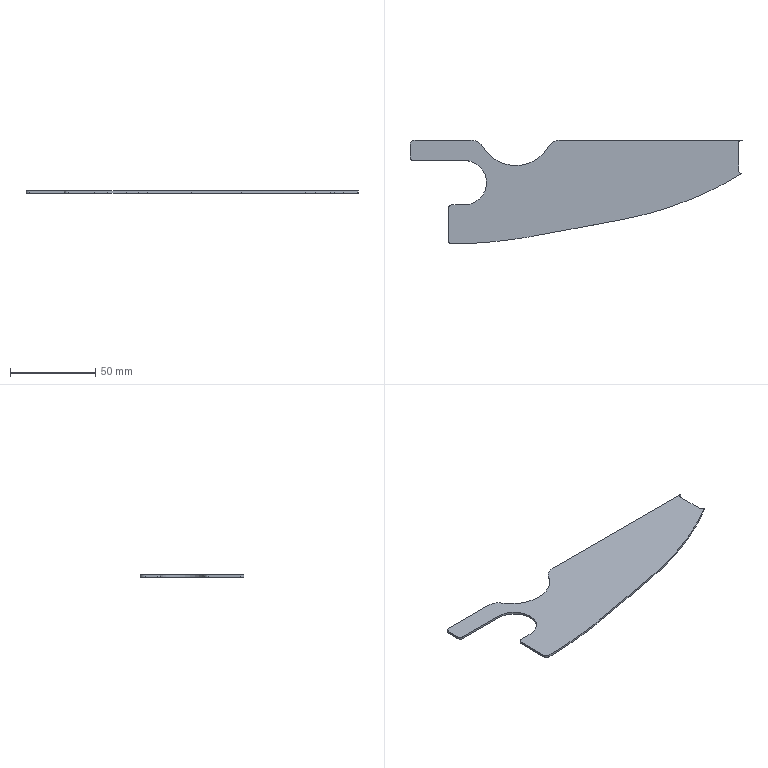Part | STEP file | gslz 2016.10.28-13_id234_x_t | 1 solid | 32 faces | box 195 x 61.022 x 1.25 mm | volume 9258 mm3 | plane 20 | cylinder 12 | commonest cylinder face diameters 4 x5 16 x2 6 x1 26 x1 45 x1 300 x1